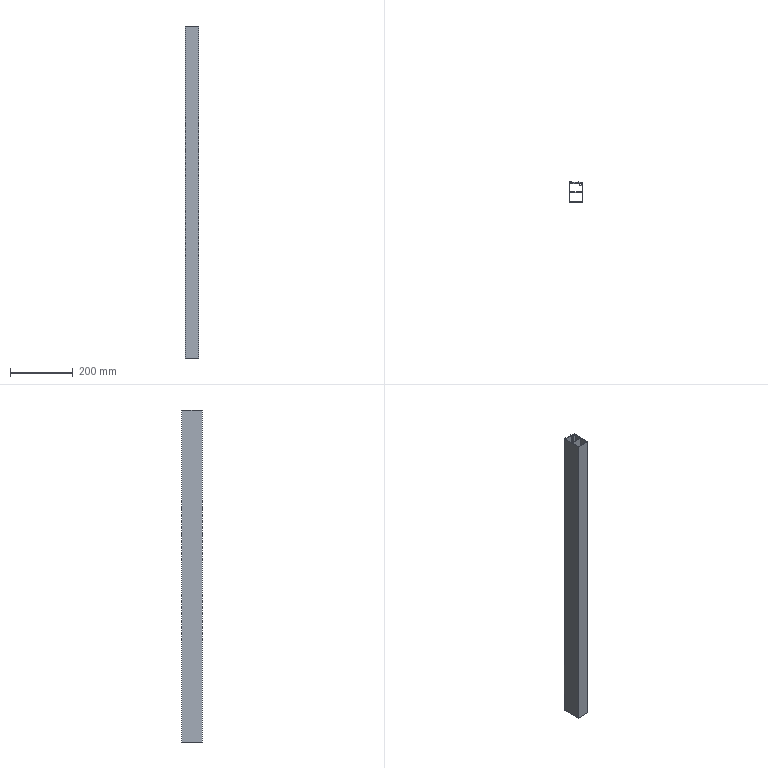Part | SolidWorks | features Extrusion 1 | 1 solid | 34 faces | box 43 x 64.5 x 1060 mm | volume 529141 mm3 | plane 34
STEP:
#1=CARTESIAN_POINT('',(13.5,31.,530.));
#2=VERTEX_POINT('',#1);
#3=CARTESIAN_POINT('',(9.5,31.,530.));
#4=VERTEX_POINT('',#3);
#5=CARTESIAN_POINT('',(13.5,31.,530.));
#6=DIRECTION('',(-1.,0.,0.));
#7=VECTOR('',#6,1000.);
#8=LINE('',#5,#7);
#9=EDGE_CURVE('',#2,#4,#8,.T.);
#10=ORIENTED_EDGE('',*,*,#9,.T.);
#11=CARTESIAN_POINT('',(9.5,33.5,530.));
#12=VERTEX_POINT('',#11);
#13=CARTESIAN_POINT('',(9.5,33.5,530.));
#14=DIRECTION('',(0.,1.,0.));
#15=VECTOR('',#14,1000.);
#16=LINE('',#13,#15);
#17=EDGE_CURVE('',#4,#12,#16,.T.);
#18=ORIENTED_EDGE('',*,*,#17,.T.);
#19=CARTESIAN_POINT('',(8.,33.5,530.));
#20=VERTEX_POINT('',#19);
#21=CARTESIAN_POINT('',(8.,33.5,530.));
#22=DIRECTION('',(-1.,0.,0.));
#23=VECTOR('',#22,1000.);
#24=LINE('',#21,#23);
#25=EDGE_CURVE('',#12,#20,#24,.T.);
#26=ORIENTED_EDGE('',*,*,#25,.T.);
#27=CARTESIAN_POINT('',(8.,31.,530.));
#28=VERTEX_POINT('',#27);
#29=CARTESIAN_POINT('',(8.,33.5,530.));
#30=DIRECTION('',(0.,-1.,0.));
#31=VECTOR('',#30,1000.);
#32=LINE('',#29,#31);
#33=EDGE_CURVE('',#20,#28,#32,.T.);
#34=ORIENTED_EDGE('',*,*,#33,.T.);
#35=CARTESIAN_POINT('',(-14.,31.,530.));
#36=VERTEX_POINT('',#35);
#37=CARTESIAN_POINT('',(8.,31.,530.));
#38=DIRECTION('',(-1.,0.,0.));
#39=VECTOR('',#38,1000.);
#40=LINE('',#37,#39);
#41=EDGE_CURVE('',#28,#36,#40,.T.);
#42=ORIENTED_EDGE('',*,*,#41,.T.);
#43=CARTESIAN_POINT('',(-14.,33.5,530.));
#44=VERTEX_POINT('',#43);
#45=CARTESIAN_POINT('',(-14.,33.5,530.));
#46=DIRECTION('',(0.,1.,0.));
#47=VECTOR('',#46,1000.);
#48=LINE('',#45,#47);
#49=EDGE_CURVE('',#36,#44,#48,.T.);
#50=ORIENTED_EDGE('',*,*,#49,.T.);
#51=CARTESIAN_POINT('',(-15.5,33.5,530.));
#52=VERTEX_POINT('',#51);
#53=CARTESIAN_POINT('',(-15.5,33.5,530.));
#54=DIRECTION('',(-1.,0.,0.));
#55=VECTOR('',#54,1000.);
#56=LINE('',#53,#55);
#57=EDGE_CURVE('',#44,#52,#56,.T.);
#58=ORIENTED_EDGE('',*,*,#57,.T.);
#59=CARTESIAN_POINT('',(-15.5,31.,530.));
#60=VERTEX_POINT('',#59);
#61=CARTESIAN_POINT('',(-15.5,33.5,530.));
#62=DIRECTION('',(0.,-1.,0.));
#63=VECTOR('',#62,1000.);
#64=LINE('',#61,#63);
#65=EDGE_CURVE('',#52,#60,#64,.T.);
#66=ORIENTED_EDGE('',*,*,#65,.T.);
#67=CARTESIAN_POINT('',(-19.,31.,530.));
#68=VERTEX_POINT('',#67);
#69=CARTESIAN_POINT('',(-15.5,31.,530.));
#70=DIRECTION('',(-1.,0.,0.));
#71=VECTOR('',#70,1000.);
#72=LINE('',#69,#71);
#73=EDGE_CURVE('',#60,#68,#72,.T.);
#74=ORIENTED_EDGE('',*,*,#73,.T.);
#75=CARTESIAN_POINT('',(-19.,33.5,530.));
#76=VERTEX_POINT('',#75);
#77=CARTESIAN_POINT('',(-19.,31.,530.));
#78=DIRECTION('',(0.,1.,0.));
#79=VECTOR('',#78,1000.);
#80=LINE('',#77,#79);
#81=EDGE_CURVE('',#68,#76,#80,.T.);
#82=ORIENTED_EDGE('',*,*,#81,.T.);
#83=CARTESIAN_POINT('',(-21.5,33.5,530.));
#84=VERTEX_POINT('',#83);
#85=CARTESIAN_POINT('',(-19.,33.5,530.));
#86=DIRECTION('',(-1.,0.,0.));
#87=VECTOR('',#86,1000.);
#88=LINE('',#85,#87);
#89=EDGE_CURVE('',#76,#84,#88,.T.);
#90=ORIENTED_EDGE('',*,*,#89,.T.);
#91=CARTESIAN_POINT('',(-21.5,-31.,530.));
#92=VERTEX_POINT('',#91);
#93=CARTESIAN_POINT('',(-21.5,33.5,530.));
#94=DIRECTION('',(0.,-1.,0.));
#95=VECTOR('',#94,1000.);
#96=LINE('',#93,#95);
#97=EDGE_CURVE('',#84,#92,#96,.T.);
#98=ORIENTED_EDGE('',*,*,#97,.T.);
#99=CARTESIAN_POINT('',(21.5,-31.,530.));
#100=VERTEX_POINT('',#99);
#101=CARTESIAN_POINT('',(21.5,-31.,530.));
#102=DIRECTION('',(1.,0.,0.));
#103=VECTOR('',#102,1000.);
#104=LINE('',#101,#103);
#105=EDGE_CURVE('',#92,#100,#104,.T.);
#106=ORIENTED_EDGE('',*,*,#105,.T.);
#107=CARTESIAN_POINT('',(21.5,31.,530.));
#108=VERTEX_POINT('',#107);
#109=CARTESIAN_POINT('',(21.5,-31.,530.));
#110=DIRECTION('',(0.,1.,0.));
#111=VECTOR('',#110,1000.);
#112=LINE('',#109,#111);
#113=EDGE_CURVE('',#100,#108,#112,.T.);
#114=ORIENTED_EDGE('',*,*,#113,.T.);
#115=CARTESIAN_POINT('',(17.5,31.,530.));
#116=VERTEX_POINT('',#115);
#117=CARTESIAN_POINT('',(21.5,31.,530.));
#118=DIRECTION('',(-1.,0.,0.));
#119=VECTOR('',#118,1000.);
#120=LINE('',#117,#119);
#121=EDGE_CURVE('',#108,#116,#120,.T.);
#122=ORIENTED_EDGE('',*,*,#121,.T.);
#123=CARTESIAN_POINT('',(17.5,29.,530.));
#124=VERTEX_POINT('',#123);
#125=CARTESIAN_POINT('',(17.5,31.,530.));
#126=DIRECTION('',(0.,-1.,0.));
#127=VECTOR('',#126,1000.);
#128=LINE('',#125,#127);
#129=EDGE_CURVE('',#116,#124,#128,.T.);
#130=ORIENTED_EDGE('',*,*,#129,.T.);
#131=CARTESIAN_POINT('',(19.5,29.,530.));
#132=VERTEX_POINT('',#131);
#133=CARTESIAN_POINT('',(19.5,29.,530.));
#134=DIRECTION('',(1.,0.,0.));
#135=VECTOR('',#134,1000.);
#136=LINE('',#133,#135);
#137=EDGE_CURVE('',#124,#132,#136,.T.);
#138=ORIENTED_EDGE('',*,*,#137,.T.);
#139=CARTESIAN_POINT('',(19.5,24.,530.));
#140=VERTEX_POINT('',#139);
#141=CARTESIAN_POINT('',(19.5,24.,530.));
#142=DIRECTION('',(0.,-1.,0.));
#143=VECTOR('',#142,1000.);
#144=LINE('',#141,#143);
#145=EDGE_CURVE('',#132,#140,#144,.T.);
#146=ORIENTED_EDGE('',*,*,#145,.T.);
#147=CARTESIAN_POINT('',(12.5,24.,530.));
#148=VERTEX_POINT('',#147);
#149=CARTESIAN_POINT('',(12.5,24.,530.));
#150=DIRECTION('',(-1.,0.,0.));
#151=VECTOR('',#150,1000.);
#152=LINE('',#149,#151);
#153=EDGE_CURVE('',#140,#148,#152,.T.);
#154=ORIENTED_EDGE('',*,*,#153,.T.);
#155=CARTESIAN_POINT('',(12.5,29.,530.));
#156=VERTEX_POINT('',#155);
#157=CARTESIAN_POINT('',(12.5,29.,530.));
#158=DIRECTION('',(0.,1.,0.));
#159=VECTOR('',#158,1000.);
#160=LINE('',#157,#159);
#161=EDGE_CURVE('',#148,#156,#160,.T.);
#162=ORIENTED_EDGE('',*,*,#161,.T.);
#163=CARTESIAN_POINT('',(13.5,29.,530.));
#164=VERTEX_POINT('',#163);
#165=CARTESIAN_POINT('',(13.5,29.,530.));
#166=DIRECTION('',(1.,0.,0.));
#167=VECTOR('',#166,1000.);
#168=LINE('',#165,#167);
#169=EDGE_CURVE('',#156,#164,#168,.T.);
#170=ORIENTED_EDGE('',*,*,#169,.T.);
#171=CARTESIAN_POINT('',(13.5,31.,530.));
#172=DIRECTION('',(0.,1.,0.));
#173=VECTOR('',#172,1000.);
#174=LINE('',#171,#173);
#175=EDGE_CURVE('',#164,#2,#174,.T.);
#176=ORIENTED_EDGE('',*,*,#175,.T.);
#177=EDGE_LOOP('',(#10,#18,#26,#34,#42,#50,#58,#66,#74,#82,#90,#98,#106,#114,#122,#130,#138,#146,#154,#162,#170,#176));
#178=FACE_OUTER_BOUND('',#177,.T.);
#179=CARTESIAN_POINT('',(19.5,22.4,530.));
#180=VERTEX_POINT('',#179);
#181=CARTESIAN_POINT('',(10.1,22.4,530.));
#182=VERTEX_POINT('',#181);
#183=CARTESIAN_POINT('',(10.1,22.4,530.));
#184=DIRECTION('',(-1.,0.,0.));
#185=VECTOR('',#184,1000.);
#186=LINE('',#183,#185);
#187=EDGE_CURVE('',#180,#182,#186,.T.);
#188=ORIENTED_EDGE('',*,*,#187,.F.);
#189=CARTESIAN_POINT('',(19.5,0.8,530.));
#190=VERTEX_POINT('',#189);
#191=CARTESIAN_POINT('',(19.5,0.8,530.));
#192=DIRECTION('',(0.,1.,0.));
#193=VECTOR('',#192,1000.);
#194=LINE('',#191,#193);
#195=EDGE_CURVE('',#190,#180,#194,.T.);
#196=ORIENTED_EDGE('',*,*,#195,.F.);
#197=CARTESIAN_POINT('',(-19.5,0.8,530.));
#198=VERTEX_POINT('',#197);
#199=CARTESIAN_POINT('',(19.5,0.8,530.));
#200=DIRECTION('',(1.,0.,0.));
#201=VECTOR('',#200,1000.);
#202=LINE('',#199,#201);
#203=EDGE_CURVE('',#198,#190,#202,.T.);
#204=ORIENTED_EDGE('',*,*,#203,.F.);
#205=CARTESIAN_POINT('',(-19.5,29.,530.));
#206=VERTEX_POINT('',#205);
#207=CARTESIAN_POINT('',(-19.5,0.8,530.));
#208=DIRECTION('',(0.,-1.,0.));
#209=VECTOR('',#208,1000.);
#210=LINE('',#207,#209);
#211=EDGE_CURVE('',#206,#198,#210,.T.);
#212=ORIENTED_EDGE('',*,*,#211,.F.);
#213=CARTESIAN_POINT('',(10.1,29.,530.));
#214=VERTEX_POINT('',#213);
#215=CARTESIAN_POINT('',(10.1,29.,530.));
#216=DIRECTION('',(-1.,0.,0.));
#217=VECTOR('',#216,1000.);
#218=LINE('',#215,#217);
#219=EDGE_CURVE('',#214,#206,#218,.T.);
#220=ORIENTED_EDGE('',*,*,#219,.F.);
#221=CARTESIAN_POINT('',(10.1,29.,530.));
#222=DIRECTION('',(0.,1.,0.));
#223=VECTOR('',#222,1000.);
#224=LINE('',#221,#223);
#225=EDGE_CURVE('',#182,#214,#224,.T.);
#226=ORIENTED_EDGE('',*,*,#225,.F.);
#227=EDGE_LOOP('',(#188,#196,#204,#212,#220,#226));
#228=FACE_BOUND('',#227,.T.);
#229=CARTESIAN_POINT('',(19.5,-29.,530.));
#230=VERTEX_POINT('',#229);
#231=CARTESIAN_POINT('',(19.5,-0.8,530.));
#232=VERTEX_POINT('',#231);
#233=CARTESIAN_POINT('',(19.5,-29.,530.));
#234=DIRECTION('',(0.,1.,0.));
#235=VECTOR('',#234,1000.);
#236=LINE('',#233,#235);
#237=EDGE_CURVE('',#230,#232,#236,.T.);
#238=ORIENTED_EDGE('',*,*,#237,.F.);
#239=CARTESIAN_POINT('',(-19.5,-29.,530.));
#240=VERTEX_POINT('',#239);
#241=CARTESIAN_POINT('',(19.5,-29.,530.));
#242=DIRECTION('',(1.,0.,0.));
#243=VECTOR('',#242,1000.);
#244=LINE('',#241,#243);
#245=EDGE_CURVE('',#240,#230,#244,.T.);
#246=ORIENTED_EDGE('',*,*,#245,.F.);
#247=CARTESIAN_POINT('',(-19.5,-0.8,530.));
#248=VERTEX_POINT('',#247);
#249=CARTESIAN_POINT('',(-19.5,-29.,530.));
#250=DIRECTION('',(0.,-1.,0.));
#251=VECTOR('',#250,1000.);
#252=LINE('',#249,#251);
#253=EDGE_CURVE('',#248,#240,#252,.T.);
#254=ORIENTED_EDGE('',*,*,#253,.F.);
#255=CARTESIAN_POINT('',(19.5,-0.8,530.));
#256=DIRECTION('',(-1.,0.,0.));
#257=VECTOR('',#256,1000.);
#258=LINE('',#255,#257);
#259=EDGE_CURVE('',#232,#248,#258,.T.);
#260=ORIENTED_EDGE('',*,*,#259,.F.);
#261=EDGE_LOOP('',(#238,#246,#254,#260));
#262=FACE_BOUND('',#261,.T.);
#263=CARTESIAN_POINT('',(0.,0.,530.));
#264=DIRECTION('',(0.,0.,1.));
#265=DIRECTION('',(1.,0.,0.));
#266=AXIS2_PLACEMENT_3D('',#263,#264,#265);
#267=PLANE('',#266);
#268=ADVANCED_FACE('',(#178,#228,#262),#267,.T.);
#269=CARTESIAN_POINT('',(19.5,0.8,-530.));
#270=VERTEX_POINT('',#269);
#271=CARTESIAN_POINT('',(19.5,22.4,-530.));
#272=VERTEX_POINT('',#271);
#273=CARTESIAN_POINT('',(19.5,0.8,-530.));
#274=DIRECTION('',(0.,1.,0.));
#275=VECTOR('',#274,1000.);
#276=LINE('',#273,#275);
#277=EDGE_CURVE('',#270,#272,#276,.T.);
#278=ORIENTED_EDGE('',*,*,#277,.T.);
#279=CARTESIAN_POINT('',(10.1,22.4,-530.));
#280=VERTEX_POINT('',#279);
#281=CARTESIAN_POINT('',(10.1,22.4,-530.));
#282=DIRECTION('',(-1.,0.,0.));
#283=VECTOR('',#282,1000.);
#284=LINE('',#281,#283);
#285=EDGE_CURVE('',#272,#280,#284,.T.);
#286=ORIENTED_EDGE('',*,*,#285,.T.);
#287=CARTESIAN_POINT('',(10.1,29.,-530.));
#288=VERTEX_POINT('',#287);
#289=CARTESIAN_POINT('',(10.1,29.,-530.));
#290=DIRECTION('',(0.,1.,0.));
#291=VECTOR('',#290,1000.);
#292=LINE('',#289,#291);
#293=EDGE_CURVE('',#280,#288,#292,.T.);
#294=ORIENTED_EDGE('',*,*,#293,.T.);
#295=CARTESIAN_POINT('',(-19.5,29.,-530.));
#296=VERTEX_POINT('',#295);
#297=CARTESIAN_POINT('',(10.1,29.,-530.));
#298=DIRECTION('',(-1.,0.,0.));
#299=VECTOR('',#298,1000.);
#300=LINE('',#297,#299);
#301=EDGE_CURVE('',#288,#296,#300,.T.);
#302=ORIENTED_EDGE('',*,*,#301,.T.);
#303=CARTESIAN_POINT('',(-19.5,0.8,-530.));
#304=VERTEX_POINT('',#303);
#305=CARTESIAN_POINT('',(-19.5,0.8,-530.));
#306=DIRECTION('',(0.,-1.,0.));
#307=VECTOR('',#306,1000.);
#308=LINE('',#305,#307);
#309=EDGE_CURVE('',#296,#304,#308,.T.);
#310=ORIENTED_EDGE('',*,*,#309,.T.);
#311=CARTESIAN_POINT('',(19.5,0.8,-530.));
#312=DIRECTION('',(1.,0.,0.));
#313=VECTOR('',#312,1000.);
#314=LINE('',#311,#313);
#315=EDGE_CURVE('',#304,#270,#314,.T.);
#316=ORIENTED_EDGE('',*,*,#315,.T.);
#317=EDGE_LOOP('',(#278,#286,#294,#302,#310,#316));
#318=FACE_BOUND('',#317,.T.);
#319=CARTESIAN_POINT('',(13.5,31.,-530.));
#320=VERTEX_POINT('',#319);
#321=CARTESIAN_POINT('',(9.5,31.,-530.));
#322=VERTEX_POINT('',#321);
#323=CARTESIAN_POINT('',(13.5,31.,-530.));
#324=DIRECTION('',(-1.,0.,0.));
#325=VECTOR('',#324,1000.);
#326=LINE('',#323,#325);
#327=EDGE_CURVE('',#320,#322,#326,.T.);
#328=ORIENTED_EDGE('',*,*,#327,.F.);
#329=CARTESIAN_POINT('',(13.5,29.,-530.));
#330=VERTEX_POINT('',#329);
#331=CARTESIAN_POINT('',(13.5,31.,-530.));
#332=DIRECTION('',(0.,1.,0.));
#333=VECTOR('',#332,1000.);
#334=LINE('',#331,#333);
#335=EDGE_CURVE('',#330,#320,#334,.T.);
#336=ORIENTED_EDGE('',*,*,#335,.F.);
#337=CARTESIAN_POINT('',(12.5,29.,-530.));
#338=VERTEX_POINT('',#337);
#339=CARTESIAN_POINT('',(13.5,29.,-530.));
#340=DIRECTION('',(1.,0.,0.));
#341=VECTOR('',#340,1000.);
#342=LINE('',#339,#341);
#343=EDGE_CURVE('',#338,#330,#342,.T.);
#344=ORIENTED_EDGE('',*,*,#343,.F.);
#345=CARTESIAN_POINT('',(12.5,24.,-530.));
#346=VERTEX_POINT('',#345);
#347=CARTESIAN_POINT('',(12.5,29.,-530.));
#348=DIRECTION('',(0.,1.,0.));
#349=VECTOR('',#348,1000.);
#350=LINE('',#347,#349);
#351=EDGE_CURVE('',#346,#338,#350,.T.);
#352=ORIENTED_EDGE('',*,*,#351,.F.);
#353=CARTESIAN_POINT('',(19.5,24.,-530.));
#354=VERTEX_POINT('',#353);
#355=CARTESIAN_POINT('',(12.5,24.,-530.));
#356=DIRECTION('',(-1.,0.,0.));
#357=VECTOR('',#356,1000.);
#358=LINE('',#355,#357);
#359=EDGE_CURVE('',#354,#346,#358,.T.);
#360=ORIENTED_EDGE('',*,*,#359,.F.);
#361=CARTESIAN_POINT('',(19.5,29.,-530.));
#362=VERTEX_POINT('',#361);
#363=CARTESIAN_POINT('',(19.5,24.,-530.));
#364=DIRECTION('',(0.,-1.,0.));
#365=VECTOR('',#364,1000.);
#366=LINE('',#363,#365);
#367=EDGE_CURVE('',#362,#354,#366,.T.);
#368=ORIENTED_EDGE('',*,*,#367,.F.);
#369=CARTESIAN_POINT('',(17.5,29.,-530.));
#370=VERTEX_POINT('',#369);
#371=CARTESIAN_POINT('',(19.5,29.,-530.));
#372=DIRECTION('',(1.,0.,0.));
#373=VECTOR('',#372,1000.);
#374=LINE('',#371,#373);
#375=EDGE_CURVE('',#370,#362,#374,.T.);
#376=ORIENTED_EDGE('',*,*,#375,.F.);
#377=CARTESIAN_POINT('',(17.5,31.,-530.));
#378=VERTEX_POINT('',#377);
#379=CARTESIAN_POINT('',(17.5,31.,-530.));
#380=DIRECTION('',(0.,-1.,0.));
#381=VECTOR('',#380,1000.);
#382=LINE('',#379,#381);
#383=EDGE_CURVE('',#378,#370,#382,.T.);
#384=ORIENTED_EDGE('',*,*,#383,.F.);
#385=CARTESIAN_POINT('',(21.5,31.,-530.));
#386=VERTEX_POINT('',#385);
#387=CARTESIAN_POINT('',(21.5,31.,-530.));
#388=DIRECTION('',(-1.,0.,0.));
#389=VECTOR('',#388,1000.);
#390=LINE('',#387,#389);
#391=EDGE_CURVE('',#386,#378,#390,.T.);
#392=ORIENTED_EDGE('',*,*,#391,.F.);
#393=CARTESIAN_POINT('',(21.5,-31.,-530.));
#394=VERTEX_POINT('',#393);
#395=CARTESIAN_POINT('',(21.5,-31.,-530.));
#396=DIRECTION('',(0.,1.,0.));
#397=VECTOR('',#396,1000.);
#398=LINE('',#395,#397);
#399=EDGE_CURVE('',#394,#386,#398,.T.);
#400=ORIENTED_EDGE('',*,*,#399,.F.);
#401=CARTESIAN_POINT('',(-21.5,-31.,-530.));
#402=VERTEX_POINT('',#401);
#403=CARTESIAN_POINT('',(21.5,-31.,-530.));
#404=DIRECTION('',(1.,0.,0.));
#405=VECTOR('',#404,1000.);
#406=LINE('',#403,#405);
#407=EDGE_CURVE('',#402,#394,#406,.T.);
#408=ORIENTED_EDGE('',*,*,#407,.F.);
#409=CARTESIAN_POINT('',(-21.5,33.5,-530.));
#410=VERTEX_POINT('',#409);
#411=CARTESIAN_POINT('',(-21.5,-31.,-530.));
#412=DIRECTION('',(0.,-1.,0.));
#413=VECTOR('',#412,1000.);
#414=LINE('',#411,#413);
#415=EDGE_CURVE('',#410,#402,#414,.T.);
#416=ORIENTED_EDGE('',*,*,#415,.F.);
#417=CARTESIAN_POINT('',(-19.,33.5,-530.));
#418=VERTEX_POINT('',#417);
#419=CARTESIAN_POINT('',(-19.,33.5,-530.));
#420=DIRECTION('',(-1.,0.,0.));
#421=VECTOR('',#420,1000.);
#422=LINE('',#419,#421);
#423=EDGE_CURVE('',#418,#410,#422,.T.);
#424=ORIENTED_EDGE('',*,*,#423,.F.);
#425=CARTESIAN_POINT('',(-19.,31.,-530.));
#426=VERTEX_POINT('',#425);
#427=CARTESIAN_POINT('',(-19.,31.,-530.));
#428=DIRECTION('',(0.,1.,0.));
#429=VECTOR('',#428,1000.);
#430=LINE('',#427,#429);
#431=EDGE_CURVE('',#426,#418,#430,.T.);
#432=ORIENTED_EDGE('',*,*,#431,.F.);
#433=CARTESIAN_POINT('',(-15.5,31.,-530.));
#434=VERTEX_POINT('',#433);
#435=CARTESIAN_POINT('',(-15.5,31.,-530.));
#436=DIRECTION('',(-1.,0.,0.));
#437=VECTOR('',#436,1000.);
#438=LINE('',#435,#437);
#439=EDGE_CURVE('',#434,#426,#438,.T.);
#440=ORIENTED_EDGE('',*,*,#439,.F.);
#441=CARTESIAN_POINT('',(-15.5,33.5,-530.));
#442=VERTEX_POINT('',#441);
#443=CARTESIAN_POINT('',(-15.5,33.5,-530.));
#444=DIRECTION('',(0.,-1.,0.));
#445=VECTOR('',#444,1000.);
#446=LINE('',#443,#445);
#447=EDGE_CURVE('',#442,#434,#446,.T.);
#448=ORIENTED_EDGE('',*,*,#447,.F.);
#449=CARTESIAN_POINT('',(-14.,33.5,-530.));
#450=VERTEX_POINT('',#449);
#451=CARTESIAN_POINT('',(-15.5,33.5,-530.));
#452=DIRECTION('',(-1.,0.,0.));
#453=VECTOR('',#452,1000.);
#454=LINE('',#451,#453);
#455=EDGE_CURVE('',#450,#442,#454,.T.);
#456=ORIENTED_EDGE('',*,*,#455,.F.);
#457=CARTESIAN_POINT('',(-14.,31.,-530.));
#458=VERTEX_POINT('',#457);
#459=CARTESIAN_POINT('',(-14.,33.5,-530.));
#460=DIRECTION('',(0.,1.,0.));
#461=VECTOR('',#460,1000.);
#462=LINE('',#459,#461);
#463=EDGE_CURVE('',#458,#450,#462,.T.);
#464=ORIENTED_EDGE('',*,*,#463,.F.);
#465=CARTESIAN_POINT('',(8.,31.,-530.));
#466=VERTEX_POINT('',#465);
#467=CARTESIAN_POINT('',(8.,31.,-530.));
#468=DIRECTION('',(-1.,0.,0.));
#469=VECTOR('',#468,1000.);
#470=LINE('',#467,#469);
#471=EDGE_CURVE('',#466,#458,#470,.T.);
#472=ORIENTED_EDGE('',*,*,#471,.F.);
#473=CARTESIAN_POINT('',(8.,33.5,-530.));
#474=VERTEX_POINT('',#473);
#475=CARTESIAN_POINT('',(8.,33.5,-530.));
#476=DIRECTION('',(0.,-1.,0.));
#477=VECTOR('',#476,1000.);
#478=LINE('',#475,#477);
#479=EDGE_CURVE('',#474,#466,#478,.T.);
#480=ORIENTED_EDGE('',*,*,#479,.F.);
#481=CARTESIAN_POINT('',(9.5,33.5,-530.));
#482=VERTEX_POINT('',#481);
#483=CARTESIAN_POINT('',(8.,33.5,-530.));
#484=DIRECTION('',(-1.,0.,0.));
#485=VECTOR('',#484,1000.);
#486=LINE('',#483,#485);
#487=EDGE_CURVE('',#482,#474,#486,.T.);
#488=ORIENTED_EDGE('',*,*,#487,.F.);
#489=CARTESIAN_POINT('',(9.5,33.5,-530.));
#490=DIRECTION('',(0.,1.,0.));
#491=VECTOR('',#490,1000.);
#492=LINE('',#489,#491);
#493=EDGE_CURVE('',#322,#482,#492,.T.);
#494=ORIENTED_EDGE('',*,*,#493,.F.);
#495=EDGE_LOOP('',(#328,#336,#344,#352,#360,#368,#376,#384,#392,#400,#408,#416,#424,#432,#440,#448,#456,#464,#472,#480,#488,#494));
#496=FACE_OUTER_BOUND('',#495,.T.);
#497=CARTESIAN_POINT('',(-19.5,-29.,-530.));
#498=VERTEX_POINT('',#497);
#499=CARTESIAN_POINT('',(19.5,-29.,-530.));
#500=VERTEX_POINT('',#499);
#501=CARTESIAN_POINT('',(19.5,-29.,-530.));
#502=DIRECTION('',(1.,0.,0.));
#503=VECTOR('',#502,1000.);
#504=LINE('',#501,#503);
#505=EDGE_CURVE('',#498,#500,#504,.T.);
#506=ORIENTED_EDGE('',*,*,#505,.T.);
#507=CARTESIAN_POINT('',(19.5,-0.8,-530.));
#508=VERTEX_POINT('',#507);
#509=CARTESIAN_POINT('',(19.5,-29.,-530.));
#510=DIRECTION('',(0.,1.,0.));
#511=VECTOR('',#510,1000.);
#512=LINE('',#509,#511);
#513=EDGE_CURVE('',#500,#508,#512,.T.);
#514=ORIENTED_EDGE('',*,*,#513,.T.);
#515=CARTESIAN_POINT('',(-19.5,-0.8,-530.));
#516=VERTEX_POINT('',#515);
#517=CARTESIAN_POINT('',(19.5,-0.8,-530.));
#518=DIRECTION('',(-1.,0.,0.));
#519=VECTOR('',#518,1000.);
#520=LINE('',#517,#519);
#521=EDGE_CURVE('',#508,#516,#520,.T.);
#522=ORIENTED_EDGE('',*,*,#521,.T.);
#523=CARTESIAN_POINT('',(-19.5,-29.,-530.));
#524=DIRECTION('',(0.,-1.,0.));
#525=VECTOR('',#524,1000.);
#526=LINE('',#523,#525);
#527=EDGE_CURVE('',#516,#498,#526,.T.);
#528=ORIENTED_EDGE('',*,*,#527,.T.);
#529=EDGE_LOOP('',(#506,#514,#522,#528));
#530=FACE_BOUND('',#529,.T.);
#531=CARTESIAN_POINT('',(0.,0.,-530.));
#532=DIRECTION('',(0.,0.,1.));
#533=DIRECTION('',(1.,0.,0.));
#534=AXIS2_PLACEMENT_3D('',#531,#532,#533);
#535=PLANE('',#534);
#536=ADVANCED_FACE('',(#318,#496,#530),#535,.F.);
#537=ORIENTED_EDGE('',*,*,#327,.T.);
#538=CARTESIAN_POINT('',(9.5,31.,530.));
#539=DIRECTION('',(0.,0.,-1.));
#540=VECTOR('',#539,1000.);
#541=LINE('',#538,#540);
#542=EDGE_CURVE('',#4,#322,#541,.T.);
#543=ORIENTED_EDGE('',*,*,#542,.F.);
#544=ORIENTED_EDGE('',*,*,#9,.F.);
#545=CARTESIAN_POINT('',(13.5,31.,530.));
#546=DIRECTION('',(0.,0.,-1.));
#547=VECTOR('',#546,1000.);
#548=LINE('',#545,#547);
#549=EDGE_CURVE('',#2,#320,#548,.T.);
#550=ORIENTED_EDGE('',*,*,#549,.T.);
#551=EDGE_LOOP('',(#537,#543,#544,#550));
#552=FACE_OUTER_BOUND('',#551,.T.);
#553=CARTESIAN_POINT('',(13.5,31.,530.));
#554=DIRECTION('',(0.,-1.,0.));
#555=DIRECTION('',(0.,0.,-1.));
#556=AXIS2_PLACEMENT_3D('',#553,#554,#555);
#557=PLANE('',#556);
#558=ADVANCED_FACE('',(#552),#557,.F.);
#559=ORIENTED_EDGE('',*,*,#493,.T.);
#560=CARTESIAN_POINT('',(9.5,33.5,530.));
#561=DIRECTION('',(0.,0.,-1.));
#562=VECTOR('',#561,1000.);
#563=LINE('',#560,#562);
#564=EDGE_CURVE('',#12,#482,#563,.T.);
#565=ORIENTED_EDGE('',*,*,#564,.F.);
#566=ORIENTED_EDGE('',*,*,#17,.F.);
#567=ORIENTED_EDGE('',*,*,#542,.T.);
#568=EDGE_LOOP('',(#559,#565,#566,#567));
#569=FACE_OUTER_BOUND('',#568,.T.);
#570=CARTESIAN_POINT('',(9.5,33.5,530.));
#571=DIRECTION('',(-1.,0.,0.));
#572=DIRECTION('',(0.,0.,1.));
#573=AXIS2_PLACEMENT_3D('',#570,#571,#572);
#574=PLANE('',#573);
#575=ADVANCED_FACE('',(#569),#574,.F.);
#576=ORIENTED_EDGE('',*,*,#487,.T.);
#577=CARTESIAN_POINT('',(8.,33.5,530.));
#578=DIRECTION('',(0.,0.,-1.));
#579=VECTOR('',#578,1000.);
#580=LINE('',#577,#579);
#581=EDGE_CURVE('',#20,#474,#580,.T.);
#582=ORIENTED_EDGE('',*,*,#581,.F.);
#583=ORIENTED_EDGE('',*,*,#25,.F.);
#584=ORIENTED_EDGE('',*,*,#564,.T.);
#585=EDGE_LOOP('',(#576,#582,#583,#584));
#586=FACE_OUTER_BOUND('',#585,.T.);
#587=CARTESIAN_POINT('',(8.,33.5,530.));
#588=DIRECTION('',(0.,-1.,0.));
#589=DIRECTION('',(0.,0.,-1.));
#590=AXIS2_PLACEMENT_3D('',#587,#588,#589);
#591=PLANE('',#590);
#592=ADVANCED_FACE('',(#586),#591,.F.);
#593=ORIENTED_EDGE('',*,*,#479,.T.);
#594=CARTESIAN_POINT('',(8.,31.,530.));
#595=DIRECTION('',(0.,0.,-1.));
#596=VECTOR('',#595,1000.);
#597=LINE('',#594,#596);
#598=EDGE_CURVE('',#28,#466,#597,.T.);
#599=ORIENTED_EDGE('',*,*,#598,.F.);
#600=ORIENTED_EDGE('',*,*,#33,.F.);
#601=ORIENTED_EDGE('',*,*,#581,.T.);
#602=EDGE_LOOP('',(#593,#599,#600,#601));
#603=FACE_OUTER_BOUND('',#602,.T.);
#604=CARTESIAN_POINT('',(8.,33.5,530.));
#605=DIRECTION('',(1.,0.,0.));
#606=DIRECTION('',(0.,0.,-1.));
#607=AXIS2_PLACEMENT_3D('',#604,#605,#606);
#608=PLANE('',#607);
#609=ADVANCED_FACE('',(#603),#608,.F.);
#610=ORIENTED_EDGE('',*,*,#471,.T.);
#611=CARTESIAN_POINT('',(-14.,31.,530.));
#612=DIRECTION('',(0.,0.,-1.));
#613=VECTOR('',#612,1000.);
#614=LINE('',#611,#613);
#615=EDGE_CURVE('',#36,#458,#614,.T.);
#616=ORIENTED_EDGE('',*,*,#615,.F.);
#617=ORIENTED_EDGE('',*,*,#41,.F.);
#618=ORIENTED_EDGE('',*,*,#598,.T.);
#619=EDGE_LOOP('',(#610,#616,#617,#618));
#620=FACE_OUTER_BOUND('',#619,.T.);
#621=CARTESIAN_POINT('',(8.,31.,530.));
#622=DIRECTION('',(0.,-1.,0.));
#623=DIRECTION('',(1.,0.,0.));
#624=AXIS2_PLACEMENT_3D('',#621,#622,#623);
#625=PLANE('',#624);
#626=ADVANCED_FACE('',(#620),#625,.F.);
#627=ORIENTED_EDGE('',*,*,#463,.T.);
#628=CARTESIAN_POINT('',(-14.,33.5,530.));
#629=DIRECTION('',(0.,0.,-1.));
#630=VECTOR('',#629,1000.);
#631=LINE('',#628,#630);
#632=EDGE_CURVE('',#44,#450,#631,.T.);
#633=ORIENTED_EDGE('',*,*,#632,.F.);
#634=ORIENTED_EDGE('',*,*,#49,.F.);
#635=ORIENTED_EDGE('',*,*,#615,.T.);
#636=EDGE_LOOP('',(#627,#633,#634,#635));
#637=FACE_OUTER_BOUND('',#636,.T.);
#638=CARTESIAN_POINT('',(-14.,33.5,530.));
#639=DIRECTION('',(-1.,0.,0.));
#640=DIRECTION('',(0.,0.,1.));
#641=AXIS2_PLACEMENT_3D('',#638,#639,#640);
#642=PLANE('',#641);
#643=ADVANCED_FACE('',(#637),#642,.F.);
#644=ORIENTED_EDGE('',*,*,#455,.T.);
#645=CARTESIAN_POINT('',(-15.5,33.5,530.));
#646=DIRECTION('',(0.,0.,-1.));
#647=VECTOR('',#646,1000.);
#648=LINE('',#645,#647);
#649=EDGE_CURVE('',#52,#442,#648,.T.);
#650=ORIENTED_EDGE('',*,*,#649,.F.);
#651=ORIENTED_EDGE('',*,*,#57,.F.);
#652=ORIENTED_EDGE('',*,*,#632,.T.);
#653=EDGE_LOOP('',(#644,#650,#651,#652));
#654=FACE_OUTER_BOUND('',#653,.T.);
#655=CARTESIAN_POINT('',(-15.5,33.5,530.));
#656=DIRECTION('',(0.,-1.,0.));
#657=DIRECTION('',(0.,0.,-1.));
#658=AXIS2_PLACEMENT_3D('',#655,#656,#657);
#659=PLANE('',#658);
#660=ADVANCED_FACE('',(#654),#659,.F.);
#661=ORIENTED_EDGE('',*,*,#447,.T.);
#662=CARTESIAN_POINT('',(-15.5,31.,530.));
#663=DIRECTION('',(0.,0.,-1.));
#664=VECTOR('',#663,1000.);
#665=LINE('',#662,#664);
#666=EDGE_CURVE('',#60,#434,#665,.T.);
#667=ORIENTED_EDGE('',*,*,#666,.F.);
#668=ORIENTED_EDGE('',*,*,#65,.F.);
#669=ORIENTED_EDGE('',*,*,#649,.T.);
#670=EDGE_LOOP('',(#661,#667,#668,#669));
#671=FACE_OUTER_BOUND('',#670,.T.);
#672=CARTESIAN_POINT('',(-15.5,33.5,530.));
#673=DIRECTION('',(1.,0.,0.));
#674=DIRECTION('',(0.,0.,-1.));
#675=AXIS2_PLACEMENT_3D('',#672,#673,#674);
#676=PLANE('',#675);
#677=ADVANCED_FACE('',(#671),#676,.F.);
#678=ORIENTED_EDGE('',*,*,#439,.T.);
#679=CARTESIAN_POINT('',(-19.,31.,530.));
#680=DIRECTION('',(0.,0.,-1.));
#681=VECTOR('',#680,1000.);
#682=LINE('',#679,#681);
#683=EDGE_CURVE('',#68,#426,#682,.T.);
#684=ORIENTED_EDGE('',*,*,#683,.F.);
#685=ORIENTED_EDGE('',*,*,#73,.F.);
#686=ORIENTED_EDGE('',*,*,#666,.T.);
#687=EDGE_LOOP('',(#678,#684,#685,#686));
#688=FACE_OUTER_BOUND('',#687,.T.);
#689=CARTESIAN_POINT('',(-15.5,31.,530.));
#690=DIRECTION('',(0.,-1.,0.));
#691=DIRECTION('',(0.,0.,-1.));
#692=AXIS2_PLACEMENT_3D('',#689,#690,#691);
#693=PLANE('',#692);
#694=ADVANCED_FACE('',(#688),#693,.F.);
#695=ORIENTED_EDGE('',*,*,#431,.T.);
#696=CARTESIAN_POINT('',(-19.,33.5,530.));
#697=DIRECTION('',(0.,0.,-1.));
#698=VECTOR('',#697,1000.);
#699=LINE('',#696,#698);
#700=EDGE_CURVE('',#76,#418,#699,.T.);
#701=ORIENTED_EDGE('',*,*,#700,.F.);
#702=ORIENTED_EDGE('',*,*,#81,.F.);
#703=ORIENTED_EDGE('',*,*,#683,.T.);
#704=EDGE_LOOP('',(#695,#701,#702,#703));
#705=FACE_OUTER_BOUND('',#704,.T.);
#706=CARTESIAN_POINT('',(-19.,31.,530.));
#707=DIRECTION('',(-1.,0.,0.));
#708=DIRECTION('',(0.,0.,1.));
#709=AXIS2_PLACEMENT_3D('',#706,#707,#708);
#710=PLANE('',#709);
#711=ADVANCED_FACE('',(#705),#710,.F.);
#712=ORIENTED_EDGE('',*,*,#423,.T.);
#713=CARTESIAN_POINT('',(-21.5,33.5,530.));
#714=DIRECTION('',(0.,0.,-1.));
#715=VECTOR('',#714,1000.);
#716=LINE('',#713,#715);
#717=EDGE_CURVE('',#84,#410,#716,.T.);
#718=ORIENTED_EDGE('',*,*,#717,.F.);
#719=ORIENTED_EDGE('',*,*,#89,.F.);
#720=ORIENTED_EDGE('',*,*,#700,.T.);
#721=EDGE_LOOP('',(#712,#718,#719,#720));
#722=FACE_OUTER_BOUND('',#721,.T.);
#723=CARTESIAN_POINT('',(-19.,33.5,530.));
#724=DIRECTION('',(0.,-1.,0.));
#725=DIRECTION('',(0.,0.,-1.));
#726=AXIS2_PLACEMENT_3D('',#723,#724,#725);
#727=PLANE('',#726);
#728=ADVANCED_FACE('',(#722),#727,.F.);
#729=ORIENTED_EDGE('',*,*,#415,.T.);
#730=CARTESIAN_POINT('',(-21.5,-31.,530.));
#731=DIRECTION('',(0.,0.,-1.));
#732=VECTOR('',#731,1000.);
#733=LINE('',#730,#732);
#734=EDGE_CURVE('',#92,#402,#733,.T.);
#735=ORIENTED_EDGE('',*,*,#734,.F.);
#736=ORIENTED_EDGE('',*,*,#97,.F.);
#737=ORIENTED_EDGE('',*,*,#717,.T.);
#738=EDGE_LOOP('',(#729,#735,#736,#737));
#739=FACE_OUTER_BOUND('',#738,.T.);
#740=CARTESIAN_POINT('',(-21.5,-31.,530.));
#741=DIRECTION('',(1.,0.,0.));
#742=DIRECTION('',(0.,0.,-1.));
#743=AXIS2_PLACEMENT_3D('',#740,#741,#742);
#744=PLANE('',#743);
#745=ADVANCED_FACE('',(#739),#744,.F.);
#746=ORIENTED_EDGE('',*,*,#407,.T.);
#747=CARTESIAN_POINT('',(21.5,-31.,530.));
#748=DIRECTION('',(0.,0.,-1.));
#749=VECTOR('',#748,1000.);
#750=LINE('',#747,#749);
#751=EDGE_CURVE('',#100,#394,#750,.T.);
#752=ORIENTED_EDGE('',*,*,#751,.F.);
#753=ORIENTED_EDGE('',*,*,#105,.F.);
#754=ORIENTED_EDGE('',*,*,#734,.T.);
#755=EDGE_LOOP('',(#746,#752,#753,#754));
#756=FACE_OUTER_BOUND('',#755,.T.);
#757=CARTESIAN_POINT('',(21.5,-31.,530.));
#758=DIRECTION('',(0.,1.,0.));
#759=DIRECTION('',(-1.,0.,0.));
#760=AXIS2_PLACEMENT_3D('',#757,#758,#759);
#761=PLANE('',#760);
#762=ADVANCED_FACE('',(#756),#761,.F.);
#763=ORIENTED_EDGE('',*,*,#399,.T.);
#764=CARTESIAN_POINT('',(21.5,31.,530.));
#765=DIRECTION('',(0.,0.,-1.));
#766=VECTOR('',#765,1000.);
#767=LINE('',#764,#766);
#768=EDGE_CURVE('',#108,#386,#767,.T.);
#769=ORIENTED_EDGE('',*,*,#768,.F.);
#770=ORIENTED_EDGE('',*,*,#113,.F.);
#771=ORIENTED_EDGE('',*,*,#751,.T.);
#772=EDGE_LOOP('',(#763,#769,#770,#771));
#773=FACE_OUTER_BOUND('',#772,.T.);
#774=CARTESIAN_POINT('',(21.5,-31.,530.));
#775=DIRECTION('',(-1.,0.,0.));
#776=DIRECTION('',(0.,0.,1.));
#777=AXIS2_PLACEMENT_3D('',#774,#775,#776);
#778=PLANE('',#777);
#779=ADVANCED_FACE('',(#773),#778,.F.);
#780=ORIENTED_EDGE('',*,*,#391,.T.);
#781=CARTESIAN_POINT('',(17.5,31.,530.));
#782=DIRECTION('',(0.,0.,-1.));
#783=VECTOR('',#782,1000.);
#784=LINE('',#781,#783);
#785=EDGE_CURVE('',#116,#378,#784,.T.);
#786=ORIENTED_EDGE('',*,*,#785,.F.);
#787=ORIENTED_EDGE('',*,*,#121,.F.);
#788=ORIENTED_EDGE('',*,*,#768,.T.);
#789=EDGE_LOOP('',(#780,#786,#787,#788));
#790=FACE_OUTER_BOUND('',#789,.T.);
#791=CARTESIAN_POINT('',(21.5,31.,530.));
#792=DIRECTION('',(0.,-1.,0.));
#793=DIRECTION('',(0.,0.,-1.));
#794=AXIS2_PLACEMENT_3D('',#791,#792,#793);
#795=PLANE('',#794);
#796=ADVANCED_FACE('',(#790),#795,.F.);
#797=ORIENTED_EDGE('',*,*,#383,.T.);
#798=CARTESIAN_POINT('',(17.5,29.,530.));
#799=DIRECTION('',(0.,0.,-1.));
#800=VECTOR('',#799,1000.);
#801=LINE('',#798,#800);
#802=EDGE_CURVE('',#124,#370,#801,.T.);
#803=ORIENTED_EDGE('',*,*,#802,.F.);
#804=ORIENTED_EDGE('',*,*,#129,.F.);
#805=ORIENTED_EDGE('',*,*,#785,.T.);
#806=EDGE_LOOP('',(#797,#803,#804,#805));
#807=FACE_OUTER_BOUND('',#806,.T.);
#808=CARTESIAN_POINT('',(17.5,31.,530.));
#809=DIRECTION('',(1.,0.,0.));
#810=DIRECTION('',(0.,0.,-1.));
#811=AXIS2_PLACEMENT_3D('',#808,#809,#810);
#812=PLANE('',#811);
#813=ADVANCED_FACE('',(#807),#812,.F.);
#814=ORIENTED_EDGE('',*,*,#375,.T.);
#815=CARTESIAN_POINT('',(19.5,29.,530.));
#816=DIRECTION('',(0.,0.,-1.));
#817=VECTOR('',#816,1000.);
#818=LINE('',#815,#817);
#819=EDGE_CURVE('',#132,#362,#818,.T.);
#820=ORIENTED_EDGE('',*,*,#819,.F.);
#821=ORIENTED_EDGE('',*,*,#137,.F.);
#822=ORIENTED_EDGE('',*,*,#802,.T.);
#823=EDGE_LOOP('',(#814,#820,#821,#822));
#824=FACE_OUTER_BOUND('',#823,.T.);
#825=CARTESIAN_POINT('',(19.5,29.,530.));
#826=DIRECTION('',(0.,1.,0.));
#827=DIRECTION('',(0.,0.,1.));
#828=AXIS2_PLACEMENT_3D('',#825,#826,#827);
#829=PLANE('',#828);
#830=ADVANCED_FACE('',(#824),#829,.F.);
#831=ORIENTED_EDGE('',*,*,#367,.T.);
#832=CARTESIAN_POINT('',(19.5,24.,530.));
#833=DIRECTION('',(0.,0.,-1.));
#834=VECTOR('',#833,1000.);
#835=LINE('',#832,#834);
#836=EDGE_CURVE('',#140,#354,#835,.T.);
#837=ORIENTED_EDGE('',*,*,#836,.F.);
#838=ORIENTED_EDGE('',*,*,#145,.F.);
#839=ORIENTED_EDGE('',*,*,#819,.T.);
#840=EDGE_LOOP('',(#831,#837,#838,#839));
#841=FACE_OUTER_BOUND('',#840,.T.);
#842=CARTESIAN_POINT('',(19.5,24.,530.));
#843=DIRECTION('',(1.,0.,0.));
#844=DIRECTION('',(0.,0.,-1.));
#845=AXIS2_PLACEMENT_3D('',#842,#843,#844);
#846=PLANE('',#845);
#847=ADVANCED_FACE('',(#841),#846,.F.);
#848=ORIENTED_EDGE('',*,*,#359,.T.);
#849=CARTESIAN_POINT('',(12.5,24.,530.));
#850=DIRECTION('',(0.,0.,-1.));
#851=VECTOR('',#850,1000.);
#852=LINE('',#849,#851);
#853=EDGE_CURVE('',#148,#346,#852,.T.);
#854=ORIENTED_EDGE('',*,*,#853,.F.);
#855=ORIENTED_EDGE('',*,*,#153,.F.);
#856=ORIENTED_EDGE('',*,*,#836,.T.);
#857=EDGE_LOOP('',(#848,#854,#855,#856));
#858=FACE_OUTER_BOUND('',#857,.T.);
#859=CARTESIAN_POINT('',(12.5,24.,530.));
#860=DIRECTION('',(0.,-1.,0.));
#861=DIRECTION('',(0.,0.,-1.));
#862=AXIS2_PLACEMENT_3D('',#859,#860,#861);
#863=PLANE('',#862);
#864=ADVANCED_FACE('',(#858),#863,.F.);
#865=ORIENTED_EDGE('',*,*,#351,.T.);
#866=CARTESIAN_POINT('',(12.5,29.,530.));
#867=DIRECTION('',(0.,0.,-1.));
#868=VECTOR('',#867,1000.);
#869=LINE('',#866,#868);
#870=EDGE_CURVE('',#156,#338,#869,.T.);
#871=ORIENTED_EDGE('',*,*,#870,.F.);
#872=ORIENTED_EDGE('',*,*,#161,.F.);
#873=ORIENTED_EDGE('',*,*,#853,.T.);
#874=EDGE_LOOP('',(#865,#871,#872,#873));
#875=FACE_OUTER_BOUND('',#874,.T.);
#876=CARTESIAN_POINT('',(12.5,29.,530.));
#877=DIRECTION('',(-1.,0.,0.));
#878=DIRECTION('',(0.,0.,1.));
#879=AXIS2_PLACEMENT_3D('',#876,#877,#878);
#880=PLANE('',#879);
#881=ADVANCED_FACE('',(#875),#880,.F.);
#882=ORIENTED_EDGE('',*,*,#343,.T.);
#883=CARTESIAN_POINT('',(13.5,29.,530.));
#884=DIRECTION('',(0.,0.,-1.));
#885=VECTOR('',#884,1000.);
#886=LINE('',#883,#885);
#887=EDGE_CURVE('',#164,#330,#886,.T.);
#888=ORIENTED_EDGE('',*,*,#887,.F.);
#889=ORIENTED_EDGE('',*,*,#169,.F.);
#890=ORIENTED_EDGE('',*,*,#870,.T.);
#891=EDGE_LOOP('',(#882,#888,#889,#890));
#892=FACE_OUTER_BOUND('',#891,.T.);
#893=CARTESIAN_POINT('',(13.5,29.,530.));
#894=DIRECTION('',(0.,1.,0.));
#895=DIRECTION('',(0.,0.,1.));
#896=AXIS2_PLACEMENT_3D('',#893,#894,#895);
#897=PLANE('',#896);
#898=ADVANCED_FACE('',(#892),#897,.F.);
#899=ORIENTED_EDGE('',*,*,#335,.T.);
#900=ORIENTED_EDGE('',*,*,#549,.F.);
#901=ORIENTED_EDGE('',*,*,#175,.F.);
#902=ORIENTED_EDGE('',*,*,#887,.T.);
#903=EDGE_LOOP('',(#899,#900,#901,#902));
#904=FACE_OUTER_BOUND('',#903,.T.);
#905=CARTESIAN_POINT('',(13.5,31.,530.));
#906=DIRECTION('',(-1.,0.,0.));
#907=DIRECTION('',(0.,0.,1.));
#908=AXIS2_PLACEMENT_3D('',#905,#906,#907);
#909=PLANE('',#908);
#910=ADVANCED_FACE('',(#904),#909,.F.);
#911=ORIENTED_EDGE('',*,*,#277,.F.);
#912=CARTESIAN_POINT('',(19.5,0.8,530.));
#913=DIRECTION('',(0.,0.,-1.));
#914=VECTOR('',#913,1000.);
#915=LINE('',#912,#914);
#916=EDGE_CURVE('',#190,#270,#915,.T.);
#917=ORIENTED_EDGE('',*,*,#916,.F.);
#918=ORIENTED_EDGE('',*,*,#195,.T.);
#919=CARTESIAN_POINT('',(19.5,22.4,530.));
#920=DIRECTION('',(0.,0.,-1.));
#921=VECTOR('',#920,1000.);
#922=LINE('',#919,#921);
#923=EDGE_CURVE('',#180,#272,#922,.T.);
#924=ORIENTED_EDGE('',*,*,#923,.T.);
#925=EDGE_LOOP('',(#911,#917,#918,#924));
#926=FACE_OUTER_BOUND('',#925,.T.);
#927=CARTESIAN_POINT('',(19.5,0.8,530.));
#928=DIRECTION('',(-1.,0.,0.));
#929=DIRECTION('',(0.,0.,1.));
#930=AXIS2_PLACEMENT_3D('',#927,#928,#929);
#931=PLANE('',#930);
#932=ADVANCED_FACE('',(#926),#931,.T.);
#933=ORIENTED_EDGE('',*,*,#285,.F.);
#934=ORIENTED_EDGE('',*,*,#923,.F.);
#935=ORIENTED_EDGE('',*,*,#187,.T.);
#936=CARTESIAN_POINT('',(10.1,22.4,530.));
#937=DIRECTION('',(0.,0.,-1.));
#938=VECTOR('',#937,1000.);
#939=LINE('',#936,#938);
#940=EDGE_CURVE('',#182,#280,#939,.T.);
#941=ORIENTED_EDGE('',*,*,#940,.T.);
#942=EDGE_LOOP('',(#933,#934,#935,#941));
#943=FACE_OUTER_BOUND('',#942,.T.);
#944=CARTESIAN_POINT('',(10.1,22.4,530.));
#945=DIRECTION('',(0.,-1.,0.));
#946=DIRECTION('',(0.,0.,-1.));
#947=AXIS2_PLACEMENT_3D('',#944,#945,#946);
#948=PLANE('',#947);
#949=ADVANCED_FACE('',(#943),#948,.T.);
#950=ORIENTED_EDGE('',*,*,#293,.F.);
#951=ORIENTED_EDGE('',*,*,#940,.F.);
#952=ORIENTED_EDGE('',*,*,#225,.T.);
#953=CARTESIAN_POINT('',(10.1,29.,530.));
#954=DIRECTION('',(0.,0.,-1.));
#955=VECTOR('',#954,1000.);
#956=LINE('',#953,#955);
#957=EDGE_CURVE('',#214,#288,#956,.T.);
#958=ORIENTED_EDGE('',*,*,#957,.T.);
#959=EDGE_LOOP('',(#950,#951,#952,#958));
#960=FACE_OUTER_BOUND('',#959,.T.);
#961=CARTESIAN_POINT('',(10.1,29.,530.));
#962=DIRECTION('',(-1.,0.,0.));
#963=DIRECTION('',(0.,0.,1.));
#964=AXIS2_PLACEMENT_3D('',#961,#962,#963);
#965=PLANE('',#964);
#966=ADVANCED_FACE('',(#960),#965,.T.);
#967=ORIENTED_EDGE('',*,*,#301,.F.);
#968=ORIENTED_EDGE('',*,*,#957,.F.);
#969=ORIENTED_EDGE('',*,*,#219,.T.);
#970=CARTESIAN_POINT('',(-19.5,29.,530.));
#971=DIRECTION('',(0.,0.,-1.));
#972=VECTOR('',#971,1000.);
#973=LINE('',#970,#972);
#974=EDGE_CURVE('',#206,#296,#973,.T.);
#975=ORIENTED_EDGE('',*,*,#974,.T.);
#976=EDGE_LOOP('',(#967,#968,#969,#975));
#977=FACE_OUTER_BOUND('',#976,.T.);
#978=CARTESIAN_POINT('',(10.1,29.,530.));
#979=DIRECTION('',(0.,-1.,0.));
#980=DIRECTION('',(0.,0.,-1.));
#981=AXIS2_PLACEMENT_3D('',#978,#979,#980);
#982=PLANE('',#981);
#983=ADVANCED_FACE('',(#977),#982,.T.);
#984=ORIENTED_EDGE('',*,*,#309,.F.);
#985=ORIENTED_EDGE('',*,*,#974,.F.);
#986=ORIENTED_EDGE('',*,*,#211,.T.);
#987=CARTESIAN_POINT('',(-19.5,0.8,530.));
#988=DIRECTION('',(0.,0.,-1.));
#989=VECTOR('',#988,1000.);
#990=LINE('',#987,#989);
#991=EDGE_CURVE('',#198,#304,#990,.T.);
#992=ORIENTED_EDGE('',*,*,#991,.T.);
#993=EDGE_LOOP('',(#984,#985,#986,#992));
#994=FACE_OUTER_BOUND('',#993,.T.);
#995=CARTESIAN_POINT('',(-19.5,0.8,530.));
#996=DIRECTION('',(1.,0.,0.));
#997=DIRECTION('',(0.,0.,-1.));
#998=AXIS2_PLACEMENT_3D('',#995,#996,#997);
#999=PLANE('',#998);
#1000=ADVANCED_FACE('',(#994),#999,.T.);
#1001=ORIENTED_EDGE('',*,*,#315,.F.);
#1002=ORIENTED_EDGE('',*,*,#991,.F.);
#1003=ORIENTED_EDGE('',*,*,#203,.T.);
#1004=ORIENTED_EDGE('',*,*,#916,.T.);
#1005=EDGE_LOOP('',(#1001,#1002,#1003,#1004));
#1006=FACE_OUTER_BOUND('',#1005,.T.);
#1007=CARTESIAN_POINT('',(19.5,0.8,530.));
#1008=DIRECTION('',(0.,1.,0.));
#1009=DIRECTION('',(-1.,0.,0.));
#1010=AXIS2_PLACEMENT_3D('',#1007,#1008,#1009);
#1011=PLANE('',#1010);
#1012=ADVANCED_FACE('',(#1006),#1011,.T.);
#1013=ORIENTED_EDGE('',*,*,#505,.F.);
#1014=CARTESIAN_POINT('',(-19.5,-29.,530.));
#1015=DIRECTION('',(0.,0.,-1.));
#1016=VECTOR('',#1015,1000.);
#1017=LINE('',#1014,#1016);
#1018=EDGE_CURVE('',#240,#498,#1017,.T.);
#1019=ORIENTED_EDGE('',*,*,#1018,.F.);
#1020=ORIENTED_EDGE('',*,*,#245,.T.);
#1021=CARTESIAN_POINT('',(19.5,-29.,530.));
#1022=DIRECTION('',(0.,0.,-1.));
#1023=VECTOR('',#1022,1000.);
#1024=LINE('',#1021,#1023);
#1025=EDGE_CURVE('',#230,#500,#1024,.T.);
#1026=ORIENTED_EDGE('',*,*,#1025,.T.);
#1027=EDGE_LOOP('',(#1013,#1019,#1020,#1026));
#1028=FACE_OUTER_BOUND('',#1027,.T.);
#1029=CARTESIAN_POINT('',(19.5,-29.,530.));
#1030=DIRECTION('',(0.,1.,0.));
#1031=DIRECTION('',(0.,0.,1.));
#1032=AXIS2_PLACEMENT_3D('',#1029,#1030,#1031);
#1033=PLANE('',#1032);
#1034=ADVANCED_FACE('',(#1028),#1033,.T.);
#1035=ORIENTED_EDGE('',*,*,#513,.F.);
#1036=ORIENTED_EDGE('',*,*,#1025,.F.);
#1037=ORIENTED_EDGE('',*,*,#237,.T.);
#1038=CARTESIAN_POINT('',(19.5,-0.8,530.));
#1039=DIRECTION('',(0.,0.,-1.));
#1040=VECTOR('',#1039,1000.);
#1041=LINE('',#1038,#1040);
#1042=EDGE_CURVE('',#232,#508,#1041,.T.);
#1043=ORIENTED_EDGE('',*,*,#1042,.T.);
#1044=EDGE_LOOP('',(#1035,#1036,#1037,#1043));
#1045=FACE_OUTER_BOUND('',#1044,.T.);
#1046=CARTESIAN_POINT('',(19.5,-29.,530.));
#1047=DIRECTION('',(-1.,0.,0.));
#1048=DIRECTION('',(0.,0.,1.));
#1049=AXIS2_PLACEMENT_3D('',#1046,#1047,#1048);
#1050=PLANE('',#1049);
#1051=ADVANCED_FACE('',(#1045),#1050,.T.);
#1052=ORIENTED_EDGE('',*,*,#521,.F.);
#1053=ORIENTED_EDGE('',*,*,#1042,.F.);
#1054=ORIENTED_EDGE('',*,*,#259,.T.);
#1055=CARTESIAN_POINT('',(-19.5,-0.8,530.));
#1056=DIRECTION('',(0.,0.,-1.));
#1057=VECTOR('',#1056,1000.);
#1058=LINE('',#1055,#1057);
#1059=EDGE_CURVE('',#248,#516,#1058,.T.);
#1060=ORIENTED_EDGE('',*,*,#1059,.T.);
#1061=EDGE_LOOP('',(#1052,#1053,#1054,#1060));
#1062=FACE_OUTER_BOUND('',#1061,.T.);
#1063=CARTESIAN_POINT('',(19.5,-0.8,530.));
#1064=DIRECTION('',(0.,-1.,0.));
#1065=DIRECTION('',(1.,0.,0.));
#1066=AXIS2_PLACEMENT_3D('',#1063,#1064,#1065);
#1067=PLANE('',#1066);
#1068=ADVANCED_FACE('',(#1062),#1067,.T.);
#1069=ORIENTED_EDGE('',*,*,#527,.F.);
#1070=ORIENTED_EDGE('',*,*,#1059,.F.);
#1071=ORIENTED_EDGE('',*,*,#253,.T.);
#1072=ORIENTED_EDGE('',*,*,#1018,.T.);
#1073=EDGE_LOOP('',(#1069,#1070,#1071,#1072));
#1074=FACE_OUTER_BOUND('',#1073,.T.);
#1075=CARTESIAN_POINT('',(-19.5,-29.,530.));
#1076=DIRECTION('',(1.,0.,0.));
#1077=DIRECTION('',(0.,0.,-1.));
#1078=AXIS2_PLACEMENT_3D('',#1075,#1076,#1077);
#1079=PLANE('',#1078);
#1080=ADVANCED_FACE('',(#1074),#1079,.T.);
#1081=CLOSED_SHELL('',(#268,#536,#558,#575,#592,#609,#626,#643,#660,#677,#694,#711,#728,#745,#762,#779,#796,#813,#830,#847,#864,#881,#898,#910,#932,#949,#966,#983,#1000,#1012,#1034,#1051,#1068,#1080));
#1082=MANIFOLD_SOLID_BREP('',#1081);
#1083=CARTESIAN_POINT('',(0.,0.,0.));
#1084=DIRECTION('',(0.,0.,1.));
#1085=DIRECTION('',(1.,0.,0.));
#1086=AXIS2_PLACEMENT_3D('',#1083,#1084,#1085);
#1087=(LENGTH_UNIT()NAMED_UNIT(*)SI_UNIT(.MILLI.,.METRE.));
#1088=UNCERTAINTY_MEASURE_WITH_UNIT(LENGTH_MEASURE(0.00001),#1087,'','');
#1089=(NAMED_UNIT(*)PLANE_ANGLE_UNIT()SI_UNIT($,.RADIAN.));
#1090=(NAMED_UNIT(*)SI_UNIT($,.STERADIAN.)SOLID_ANGLE_UNIT());
#1091=(GEOMETRIC_REPRESENTATION_CONTEXT(3)GLOBAL_UNCERTAINTY_ASSIGNED_CONTEXT((#1088))GLOBAL_UNIT_ASSIGNED_CONTEXT((#1087,#1089,#1090))REPRESENTATION_CONTEXT('',''));
#1092=ADVANCED_BREP_SHAPE_REPRESENTATION('',(#1082,#1086),#1091);